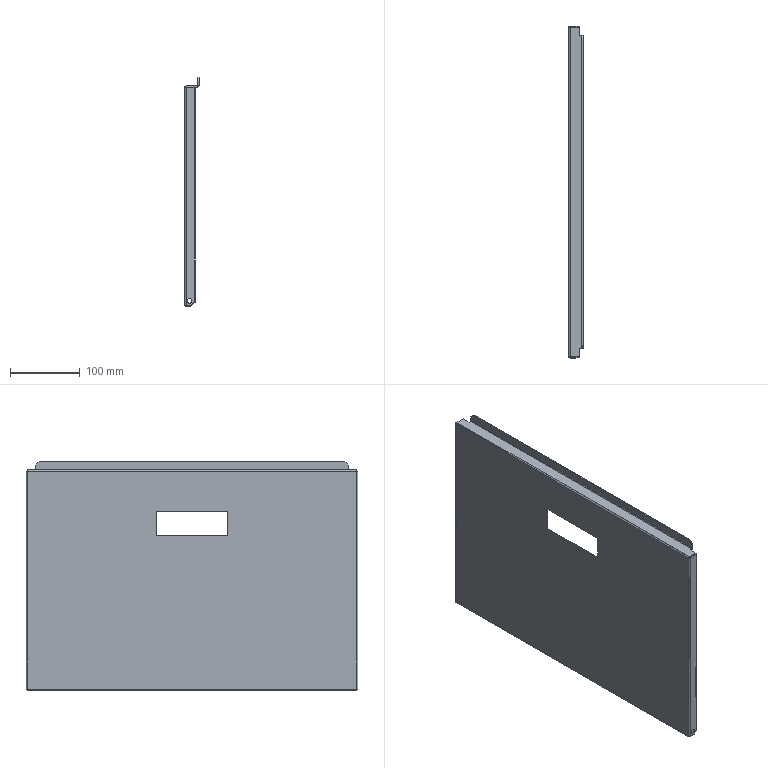Part | SolidWorks | features EdgeFlange 6, ICE 5, Chamfer 1, FlatPattern 1, SMBaseFlange 1, SheetMetal 1 | 1 solid | 96 faces | box 20.237 x 477 x 329 mm | volume 273605 mm3 | plane 76 | cylinder 20 | commonest cylinder face diameters 0.6 x6 3.6 x6 7 x4 1.473 x2 4.473 x2